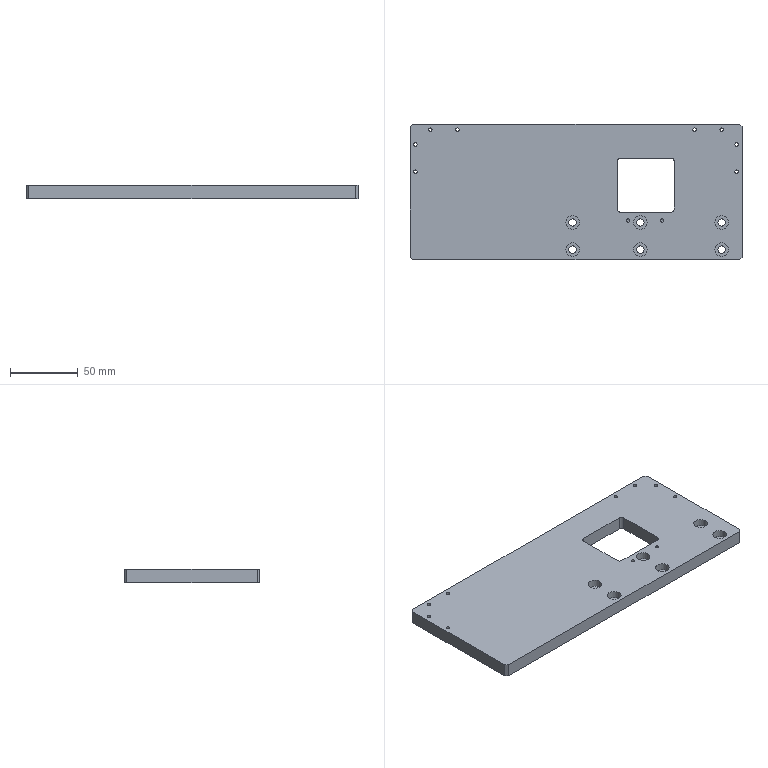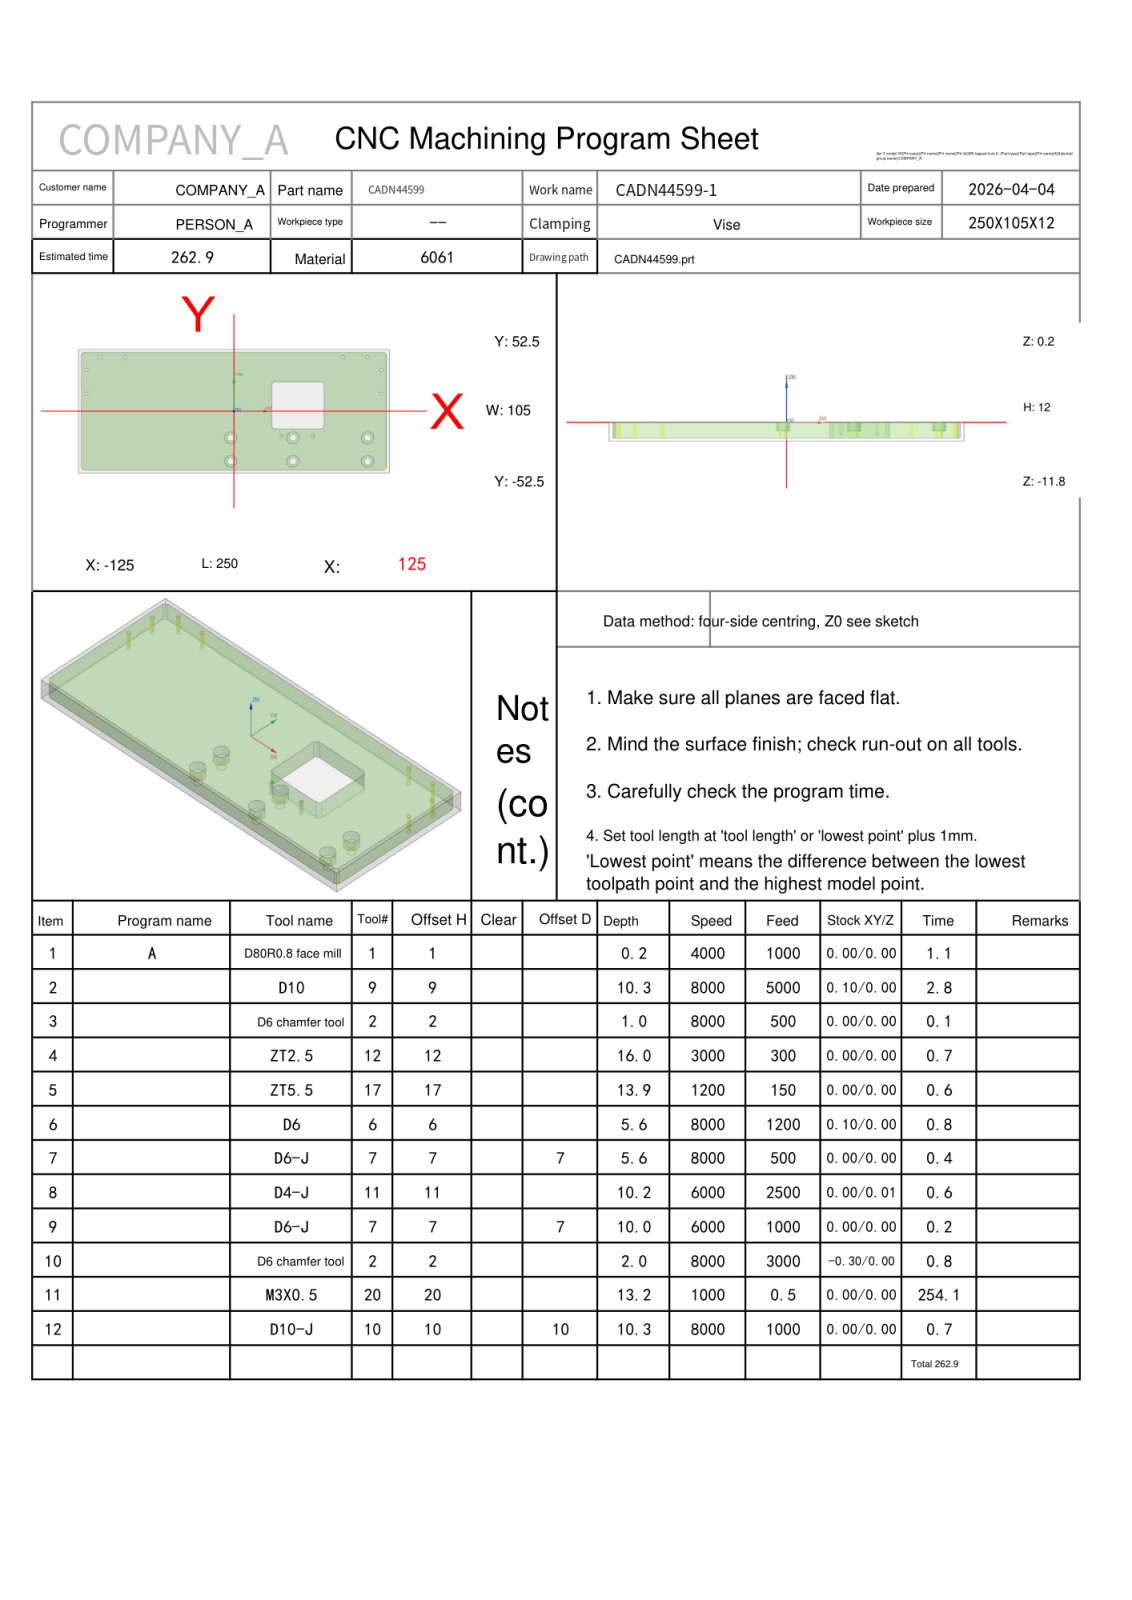NC program | NX | posted by the shop | part box 245 x 100 x 10 mm
Lines 4875 to 5259 of 5259:
N9 T07 M06
(D6-J  D=6. R=0. H=07 ce=0.00 di=0.00)
G00 G90 G54 X68.4 Y21. M03 S6000
G43 H07 Z20.
M08
Z-9.3
G01 Z-9.8 F1000.
G41 D07
X68.5
G03 X69.5 Y22. I0.0 J1.
G01 X33.5
Y-12.
X69.5
Y22.
X69.
G03 X68. Y21. I0.0 J-1.
G01 G40 Y20.9
Z-9.3
G00 Z20.
G91 G28 Z0.0
M05
M09
G91 G28 Z0.0
M01
N10 T02 M06
(D6 chamfer tool  D=6. R=0. H=02 ce=0.00 di=0.00)
G00 G90 G54 X.25 Y-52.128 M03 S8000
G43 H02 Z20.
M08
Z2.099
G01 Z-1.5 F3000.
G03 X.33 Y-51.828 I-.52 J.3
X.03 Y-51.308 I-.6 J0.0
G01 X0.0 Y-51.3
X-120.5
X-120.754 Y-51.275
X-120.997 Y-51.201
X-121.222 Y-51.081
X-121.419 Y-50.919
X-123.419 Y-48.919
X-123.581 Y-48.722
X-123.701 Y-48.497
X-123.775 Y-48.254
X-123.8 Y-48.
Y48.
X-123.775 Y48.254
X-123.701 Y48.497
X-123.581 Y48.722
X-123.419 Y48.919
X-121.419 Y50.919
X-121.222 Y51.081
X-120.997 Y51.201
X-120.754 Y51.275
X-120.5 Y51.3
X120.5
X120.754 Y51.275
X120.997 Y51.201
X121.222 Y51.081
X121.419 Y50.919
X123.419 Y48.919
X123.581 Y48.722
X123.701 Y48.497
X123.775 Y48.254
X123.8 Y48.
Y-48.
X123.775 Y-48.254
X123.701 Y-48.497
X123.581 Y-48.722
X123.419 Y-48.919
X121.419 Y-50.919
X121.222 Y-51.081
X120.997 Y-51.201
X120.754 Y-51.275
X120.5 Y-51.3
X0.0
X-.03 Y-51.308
G03 X-.33 Y-51.828 I.3 J-.52
X-.25 Y-52.128 I.6 J0.0
G01 Z2.099
G00 Z20.
X51.25 Y-12.872
Z2.099
G01 Z-1.5
G03 X51.17 Y-13.172 I.52 J-.3
X51.47 Y-13.692 I.6 J0.0
G01 X51.5 Y-13.7
X70.065
G03 X71.2 Y-12.565 I0.0 J1.135
G01 Y22.565
G03 X70.065 Y23.7 I-1.135 J0.0
G01 X32.935
G03 X31.8 Y22.565 I0.0 J-1.135
G01 Y-12.565
G03 X32.935 Y-13.7 I1.135 J0.0
G01 X51.5
X51.53 Y-13.692
G03 X51.83 Y-13.172 I-.3 J.52
X51.75 Y-12.872 I-.6 J0.0
G01 Z2.099
G00 Z20.
G00 G90 X87.5 Y46. M03 S8000
Z20.
G98 G81 X87.5 Y46. Z-1.75 R3. F500.
X107.5
X118.5 Y35.
Y15.
X63.5 Y-21.
X38.5
X-87.5 Y46.
X-107.5
X-118.5 Y35.
Y15.
G80
G00 Z20.
G00 G90 X104.846 Y-45.886 M03 S8000
Z20.
Z2.5
G01 X104.855 Y-45.894 Z2.495 F800.
X105.211 Y-46.144 Z2.337
X105.489 Y-46.304 Z2.22
X105.883 Y-46.488 Z2.062
X106.293 Y-46.63 Z1.904
X106.716 Y-46.731 Z1.746
X107.146 Y-46.788 Z1.588
X107.58 Y-46.802 Z1.43
X108.014 Y-46.772 Z1.272
X108.442 Y-46.699 Z1.114
X108.86 Y-46.582 Z.956
X109.265 Y-46.424 Z.797
X109.652 Y-46.227 Z.639
X110.016 Y-45.991 Z.481
X110.355 Y-45.719 Z.323
X110.665 Y-45.415 Z.165
X110.943 Y-45.081 Z.007
X111.186 Y-44.721 Z-.151
X111.391 Y-44.338 Z-.309
X111.556 Y-43.936 Z-.467
X111.68 Y-43.52 Z-.625
X111.762 Y-43.093 Z-.783
X111.8 Y-42.661 Z-.942
Y-42.5 Z-1.
G03 X107.5 Y-38.2 I-4.3 J0.0
X103.2 Y-42.5 I0.0 J-4.3
X107.5 Y-46.8 I4.3 J0.0
X111.8 Y-42.5 I0.0 J4.3
X111.771 Y-42.001 I-4.3 J0.0
G01 Z1.5
G00 Z20.
X104.846 Y-25.886
Z2.5
G01 X104.855 Y-25.894 Z2.495
X105.211 Y-26.144 Z2.337
X105.489 Y-26.304 Z2.22
X105.883 Y-26.488 Z2.062
X106.293 Y-26.63 Z1.904
X106.716 Y-26.731 Z1.746
X107.146 Y-26.788 Z1.588
X107.58 Y-26.802 Z1.43
X108.014 Y-26.772 Z1.272
X108.442 Y-26.699 Z1.114
X108.86 Y-26.582 Z.956
X109.265 Y-26.424 Z.797
X109.652 Y-26.227 Z.639
X110.016 Y-25.991 Z.481
X110.355 Y-25.719 Z.323
X110.665 Y-25.415 Z.165
X110.943 Y-25.081 Z.007
X111.186 Y-24.721 Z-.151
X111.391 Y-24.338 Z-.309
X111.556 Y-23.936 Z-.467
X111.68 Y-23.52 Z-.625
X111.762 Y-23.093 Z-.783
X111.8 Y-22.661 Z-.942
Y-22.5 Z-1.
G03 X107.5 Y-18.2 I-4.3 J0.0
X103.2 Y-22.5 I0.0 J-4.3
X107.5 Y-26.8 I4.3 J0.0
X111.8 Y-22.5 I0.0 J4.3
X111.771 Y-22.001 I-4.3 J0.0
G01 Z1.5
G00 Z20.
X44.846 Y-25.886
Z2.5
G01 X44.855 Y-25.894 Z2.495
X45.211 Y-26.144 Z2.337
X45.489 Y-26.304 Z2.22
X45.883 Y-26.488 Z2.062
X46.293 Y-26.63 Z1.904
X46.716 Y-26.731 Z1.746
X47.146 Y-26.788 Z1.588
X47.58 Y-26.802 Z1.43
X48.014 Y-26.772 Z1.272
X48.442 Y-26.699 Z1.114
X48.86 Y-26.582 Z.956
X49.265 Y-26.424 Z.797
X49.652 Y-26.227 Z.639
X50.016 Y-25.991 Z.481
X50.355 Y-25.719 Z.323
X50.665 Y-25.415 Z.165
X50.943 Y-25.081 Z.007
X51.186 Y-24.721 Z-.151
X51.391 Y-24.338 Z-.309
X51.556 Y-23.936 Z-.467
X51.68 Y-23.52 Z-.625
X51.762 Y-23.093 Z-.783
X51.8 Y-22.661 Z-.942
Y-22.5 Z-1.
G03 X47.5 Y-18.2 I-4.3 J0.0
X43.2 Y-22.5 I0.0 J-4.3
X47.5 Y-26.8 I4.3 J0.0
X51.8 Y-22.5 I0.0 J4.3
X51.771 Y-22.001 I-4.3 J0.0
G01 Z1.5
G00 Z20.
X44.846 Y-45.886
Z2.5
G01 X44.855 Y-45.894 Z2.495
X45.211 Y-46.144 Z2.337
X45.489 Y-46.304 Z2.22
X45.883 Y-46.488 Z2.062
X46.293 Y-46.63 Z1.904
X46.716 Y-46.731 Z1.746
X47.146 Y-46.788 Z1.588
X47.58 Y-46.802 Z1.43
X48.014 Y-46.772 Z1.272
X48.442 Y-46.699 Z1.114
X48.86 Y-46.582 Z.956
X49.265 Y-46.424 Z.797
X49.652 Y-46.227 Z.639
X50.016 Y-45.991 Z.481
X50.355 Y-45.719 Z.323
X50.665 Y-45.415 Z.165
X50.943 Y-45.081 Z.007
X51.186 Y-44.721 Z-.151
X51.391 Y-44.338 Z-.309
X51.556 Y-43.936 Z-.467
X51.68 Y-43.52 Z-.625
X51.762 Y-43.093 Z-.783
X51.8 Y-42.661 Z-.942
Y-42.5 Z-1.
G03 X47.5 Y-38.2 I-4.3 J0.0
X43.2 Y-42.5 I0.0 J-4.3
X47.5 Y-46.8 I4.3 J0.0
X51.8 Y-42.5 I0.0 J4.3
X51.771 Y-42.001 I-4.3 J0.0
G01 Z1.5
G00 Z20.
X-5.154 Y-45.886
Z2.5
G01 X-5.145 Y-45.894 Z2.495
X-4.789 Y-46.144 Z2.337
X-4.511 Y-46.304 Z2.22
X-4.117 Y-46.488 Z2.062
X-3.707 Y-46.63 Z1.904
X-3.284 Y-46.731 Z1.746
X-2.854 Y-46.788 Z1.588
X-2.42 Y-46.802 Z1.43
X-1.986 Y-46.772 Z1.272
X-1.558 Y-46.699 Z1.114
X-1.14 Y-46.582 Z.956
X-.735 Y-46.424 Z.797
X-.349 Y-46.227 Z.639
X.016 Y-45.991 Z.481
X.355 Y-45.719 Z.323
X.665 Y-45.415 Z.165
X.943 Y-45.081 Z.007
X1.186 Y-44.721 Z-.151
X1.391 Y-44.338 Z-.309
X1.556 Y-43.936 Z-.467
X1.68 Y-43.52 Z-.625
X1.762 Y-43.093 Z-.783
X1.8 Y-42.661 Z-.942
Y-42.5 Z-1.
G03 X-2.5 Y-38.2 I-4.3 J0.0
X-6.8 Y-42.5 I0.0 J-4.3
X-2.5 Y-46.8 I4.3 J0.0
X1.8 Y-42.5 I0.0 J4.3
X1.771 Y-42.001 I-4.3 J0.0
G01 Z1.5
G00 Z20.
X-5.154 Y-25.886
Z2.5
G01 X-5.145 Y-25.894 Z2.495
X-4.789 Y-26.144 Z2.337
X-4.511 Y-26.304 Z2.22
X-4.117 Y-26.488 Z2.062
X-3.707 Y-26.63 Z1.904
X-3.284 Y-26.731 Z1.746
X-2.854 Y-26.788 Z1.588
X-2.42 Y-26.802 Z1.43
X-1.986 Y-26.772 Z1.272
X-1.558 Y-26.699 Z1.114
X-1.14 Y-26.582 Z.956
X-.735 Y-26.424 Z.797
X-.349 Y-26.227 Z.639
X.016 Y-25.991 Z.481
X.355 Y-25.719 Z.323
X.665 Y-25.415 Z.165
X.943 Y-25.081 Z.007
X1.186 Y-24.721 Z-.151
X1.391 Y-24.338 Z-.309
X1.556 Y-23.936 Z-.467
X1.68 Y-23.52 Z-.625
X1.762 Y-23.093 Z-.783
X1.8 Y-22.661 Z-.942
Y-22.5 Z-1.
G03 X-2.5 Y-18.2 I-4.3 J0.0
X-6.8 Y-22.5 I0.0 J-4.3
X-2.5 Y-26.8 I4.3 J0.0
X1.8 Y-22.5 I0.0 J4.3
X1.771 Y-22.001 I-4.3 J0.0
G01 Z1.5
G00 Z20.
G91 G28 Z0.0
M05
M09
G91 G28 Z0.0
M01
N11 T20 M06
(M3X0.5 D=2.5 DR_a=180 H=20)
G00 G90 G54 X118.5 Y15. M03 S800
G43 H20 Z20.
M08
G95
G98 G84 X118.5 Y15. Z-13. R1. F.5 Q5.
Y35.
X107.5 Y46.
X87.5
X-87.5
X-107.5
X-118.5 Y35.
Y15.
G80
G94
G00 Z20.
G00 G90 X38.5 Y-21. M03 S1000
Z20.
G95
G98 G84 X38.5 Y-21. Z-6.5 R1. F.5 Q2.
X63.5
G80
G94
G00 Z20.
G91 G28 Z0.0
M05
M09
G91 G28 Z0.0
M01
N12 T10 M06
(D10-J  D=10. R=0. H=10 ce=0.00 di=0.00)
G00 G90 G54 X121.513 Y-56.116 M03 S8000
G43 H10 Z20.
M08
Z-9.6
G01 Z-10.1 F1000.
G41 D10
X121.497 Y-55.917
G03 X120.5 Y-55. I-.997 J-.083
G01 X-120.5
G02 X-124.036 Y-53.536 I0.0 J5.
G01 X-126.036 Y-51.536
G02 X-127.5 Y-48. I3.536 J3.536
G01 Y48.
G02 X-126.036 Y51.536 I5. J0.0
G01 X-124.036 Y53.536
G02 X-120.5 Y55. I3.536 J-3.536
G01 X120.5
G02 X124.036 Y53.536 I0.0 J-5.
G01 X126.036 Y51.536
G02 X127.5 Y48. I-3.536 J-3.536
G01 Y-48.
G02 X126.036 Y-51.536 I-5. J0.0
G01 X124.036 Y-53.536
G02 X120.5 Y-55. I-3.536 J3.536
G01 X120.
G03 X119. Y-56. I0.0 J-1.
G01 G40 Y-56.2
Z-9.6
G00 Z20.
M05
M09
G91 G28 Z0.0
G91 G28 Y0.0
M30
%